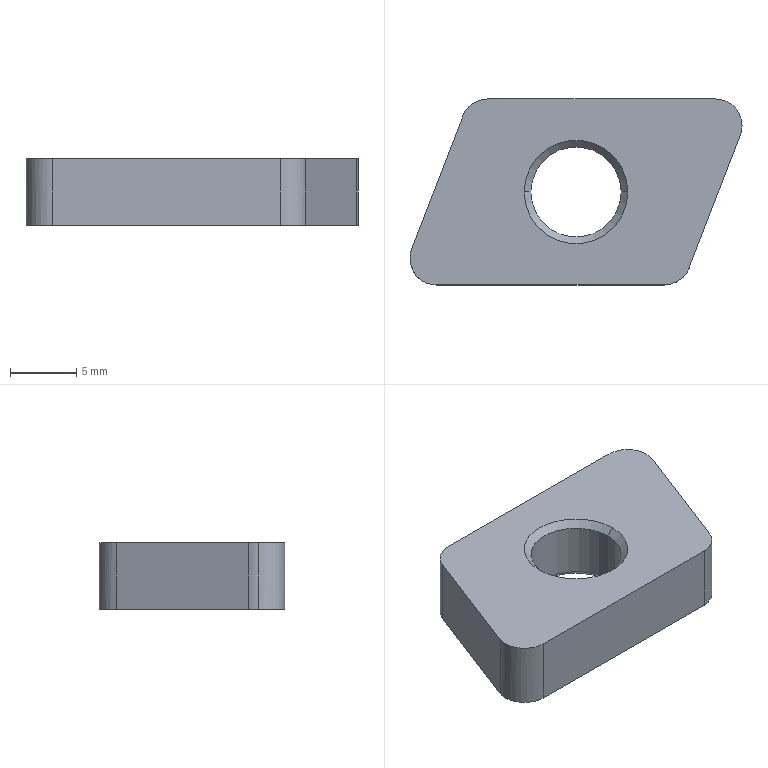Part | STEP file | 102000006924 | 1 solid | 18 faces | box 25 x 14 x 5 mm | volume 1290 mm3 | cylinder 8 | plane 6 | cone 4 | commonest cylinder face diameters 4 x6 6.8 x2
STEP:
#1=CARTESIAN_POINT('',(-2.355,42.772,4.5));
#2=VERTEX_POINT('',#1);
#3=CARTESIAN_POINT('',(4.445,42.772,4.5));
#4=VERTEX_POINT('',#3);
#5=CARTESIAN_POINT('',(1.045,42.772,4.5));
#6=DIRECTION('',(0.,0.,1.));
#7=AXIS2_PLACEMENT_3D('',#5,#6,$);
#8=CIRCLE('',#7,3.4);
#9=EDGE_CURVE('',#2,#4,#8,.T.);
#10=ORIENTED_EDGE('',*,*,#9,.F.);
#11=CARTESIAN_POINT('',(-2.855,42.772,5.));
#12=VERTEX_POINT('',#11);
#13=CARTESIAN_POINT('',(-353554.046,42.772,353556.191));
#14=DIRECTION('',(-0.7071,0.,0.7071));
#15=VECTOR('',#14,1.);
#16=LINE('',#13,#15);
#17=EDGE_CURVE('',#2,#12,#16,.T.);
#18=ORIENTED_EDGE('',*,*,#17,.T.);
#19=CARTESIAN_POINT('',(4.945,42.772,5.));
#20=VERTEX_POINT('',#19);
#21=CARTESIAN_POINT('',(1.045,42.772,5.));
#22=DIRECTION('',(0.,0.,1.));
#23=AXIS2_PLACEMENT_3D('',#21,#22,$);
#24=CIRCLE('',#23,3.9);
#25=EDGE_CURVE('',#20,#12,#24,.F.);
#26=ORIENTED_EDGE('',*,*,#25,.F.);
#27=CARTESIAN_POINT('',(353556.136,42.772,353556.191));
#28=DIRECTION('',(0.7071,0.,0.7071));
#29=VECTOR('',#28,1.);
#30=LINE('',#27,#29);
#31=EDGE_CURVE('',#4,#20,#30,.T.);
#32=ORIENTED_EDGE('',*,*,#31,.F.);
#33=EDGE_LOOP('',(#10,#18,#26,#32));
#34=FACE_OUTER_BOUND('',#33,.T.);
#35=CARTESIAN_POINT('',(1.045,42.772,4.5));
#36=DIRECTION('',(0.,0.,1.));
#37=DIRECTION('',(-1.,0.,0.));
#38=AXIS2_PLACEMENT_3D('',#35,#36,#37);
#39=CONICAL_SURFACE('',#38,3.4,0.7854);
#40=ADVANCED_FACE('',(#34),#39,.F.);
#41=CARTESIAN_POINT('',(4.445,42.772,0.5));
#42=VERTEX_POINT('',#41);
#43=CARTESIAN_POINT('',(-2.355,42.772,0.5));
#44=VERTEX_POINT('',#43);
#45=CARTESIAN_POINT('',(1.045,42.772,0.5));
#46=DIRECTION('',(0.,0.,1.));
#47=AXIS2_PLACEMENT_3D('',#45,#46,$);
#48=CIRCLE('',#47,3.4);
#49=EDGE_CURVE('',#42,#44,#48,.F.);
#50=ORIENTED_EDGE('',*,*,#49,.T.);
#51=CARTESIAN_POINT('',(-2.355,42.772,5.));
#52=DIRECTION('',(0.,0.,1.));
#53=VECTOR('',#52,1.);
#54=LINE('',#51,#53);
#55=EDGE_CURVE('',#44,#2,#54,.T.);
#56=ORIENTED_EDGE('',*,*,#55,.T.);
#57=ORIENTED_EDGE('',*,*,#9,.T.);
#58=CARTESIAN_POINT('',(4.445,42.772,5.));
#59=DIRECTION('',(0.,0.,1.));
#60=VECTOR('',#59,1.);
#61=LINE('',#58,#60);
#62=EDGE_CURVE('',#42,#4,#61,.T.);
#63=ORIENTED_EDGE('',*,*,#62,.F.);
#64=EDGE_LOOP('',(#50,#56,#57,#63));
#65=FACE_OUTER_BOUND('',#64,.T.);
#66=CARTESIAN_POINT('',(1.045,42.772,5.));
#67=DIRECTION('',(0.,0.,1.));
#68=DIRECTION('',(-1.,0.,0.));
#69=AXIS2_PLACEMENT_3D('',#66,#67,#68);
#70=CYLINDRICAL_SURFACE('',#69,3.4);
#71=ADVANCED_FACE('',(#65),#70,.F.);
#72=ORIENTED_EDGE('',*,*,#17,.F.);
#73=CARTESIAN_POINT('',(1.045,42.772,4.5));
#74=DIRECTION('',(0.,0.,1.));
#75=AXIS2_PLACEMENT_3D('',#73,#74,$);
#76=CIRCLE('',#75,3.4);
#77=EDGE_CURVE('',#4,#2,#76,.T.);
#78=ORIENTED_EDGE('',*,*,#77,.F.);
#79=ORIENTED_EDGE('',*,*,#31,.T.);
#80=CARTESIAN_POINT('',(1.045,42.772,5.));
#81=DIRECTION('',(0.,0.,1.));
#82=AXIS2_PLACEMENT_3D('',#80,#81,$);
#83=CIRCLE('',#82,3.9);
#84=EDGE_CURVE('',#12,#20,#83,.F.);
#85=ORIENTED_EDGE('',*,*,#84,.F.);
#86=EDGE_LOOP('',(#72,#78,#79,#85));
#87=FACE_OUTER_BOUND('',#86,.T.);
#88=CARTESIAN_POINT('',(1.045,42.772,4.5));
#89=DIRECTION('',(0.,0.,1.));
#90=DIRECTION('',(1.,0.,0.));
#91=AXIS2_PLACEMENT_3D('',#88,#89,#90);
#92=CONICAL_SURFACE('',#91,3.4,0.7854);
#93=ADVANCED_FACE('',(#87),#92,.F.);
#94=CARTESIAN_POINT('',(-9.455,35.772,5.));
#95=VERTEX_POINT('',#94);
#96=CARTESIAN_POINT('',(7.692,35.772,5.));
#97=VERTEX_POINT('',#96);
#98=CARTESIAN_POINT('',(-0.8816,35.772,5.));
#99=DIRECTION('',(1.,0.,0.));
#100=VECTOR('',#99,1.);
#101=LINE('',#98,#100);
#102=EDGE_CURVE('',#95,#97,#101,.T.);
#103=ORIENTED_EDGE('',*,*,#102,.T.);
#104=CARTESIAN_POINT('',(9.558,37.053,5.));
#105=VERTEX_POINT('',#104);
#106=CARTESIAN_POINT('',(7.692,35.772,5.));
#107=CARTESIAN_POINT('',(7.9,35.772,5.));
#108=CARTESIAN_POINT('',(8.107,35.799,5.));
#109=CARTESIAN_POINT('',(8.311,35.853,5.));
#110=CARTESIAN_POINT('',(8.698,36.012,5.));
#111=CARTESIAN_POINT('',(9.032,36.266,5.));
#112=CARTESIAN_POINT('',(9.182,36.413,5.));
#113=CARTESIAN_POINT('',(9.351,36.631,5.));
#114=CARTESIAN_POINT('',(9.48,36.872,5.));
#115=CARTESIAN_POINT('',(9.508,36.931,5.));
#116=CARTESIAN_POINT('',(9.534,36.991,5.));
#117=CARTESIAN_POINT('',(9.558,37.053,5.));
#118=B_SPLINE_CURVE_WITH_KNOTS('',5,(#106,#107,#108,#109,#110,#111,#112,#113,#114,#115,#116,#117),.UNSPECIFIED.,.F.,.U.,(6,3,3,6),(0.,1.47,2.939,3.402),.UNSPECIFIED.);
#119=EDGE_CURVE('',#97,#105,#118,.T.);
#120=ORIENTED_EDGE('',*,*,#119,.T.);
#121=CARTESIAN_POINT('',(13.411,47.053,5.));
#122=VERTEX_POINT('',#121);
#123=CARTESIAN_POINT('',(11.485,42.053,5.));
#124=DIRECTION('',(0.3596,0.9331,0.));
#125=VECTOR('',#124,1.);
#126=LINE('',#123,#125);
#127=EDGE_CURVE('',#105,#122,#126,.T.);
#128=ORIENTED_EDGE('',*,*,#127,.T.);
#129=CARTESIAN_POINT('',(13.545,47.772,5.));
#130=VERTEX_POINT('',#129);
#131=CARTESIAN_POINT('',(13.411,47.053,5.));
#132=CARTESIAN_POINT('',(13.464,47.19,5.));
#133=CARTESIAN_POINT('',(13.504,47.332,5.));
#134=CARTESIAN_POINT('',(13.531,47.477,5.));
#135=CARTESIAN_POINT('',(13.545,47.625,5.));
#136=CARTESIAN_POINT('',(13.545,47.772,5.));
#137=B_SPLINE_CURVE_WITH_KNOTS('',5,(#131,#132,#133,#134,#135,#136),.UNSPECIFIED.,.F.,.U.,(6,6),(0.,1.04),.UNSPECIFIED.);
#138=EDGE_CURVE('',#122,#130,#137,.T.);
#139=ORIENTED_EDGE('',*,*,#138,.T.);
#140=CARTESIAN_POINT('',(11.545,49.772,5.));
#141=VERTEX_POINT('',#140);
#142=CARTESIAN_POINT('',(13.545,47.772,5.));
#143=CARTESIAN_POINT('',(13.545,47.832,5.));
#144=CARTESIAN_POINT('',(13.543,47.893,5.));
#145=CARTESIAN_POINT('',(13.538,47.954,5.));
#146=CARTESIAN_POINT('',(13.508,48.221,5.));
#147=CARTESIAN_POINT('',(13.432,48.481,5.));
#148=CARTESIAN_POINT('',(13.348,48.674,5.));
#149=CARTESIAN_POINT('',(13.132,49.033,5.));
#150=CARTESIAN_POINT('',(12.831,49.325,5.));
#151=CARTESIAN_POINT('',(12.662,49.45,5.));
#152=CARTESIAN_POINT('',(12.346,49.627,5.));
#153=CARTESIAN_POINT('',(11.999,49.728,5.));
#154=CARTESIAN_POINT('',(11.849,49.757,5.));
#155=CARTESIAN_POINT('',(11.697,49.772,5.));
#156=CARTESIAN_POINT('',(11.545,49.772,5.));
#157=B_SPLINE_CURVE_WITH_KNOTS('',5,(#142,#143,#144,#145,#146,#147,#148,#149,#150,#151,#152,#153,#154,#155,#156),.UNSPECIFIED.,.F.,.U.,(6,3,3,3,6),(1.04,1.47,2.939,4.409,5.483),.UNSPECIFIED.);
#158=EDGE_CURVE('',#130,#141,#157,.T.);
#159=ORIENTED_EDGE('',*,*,#158,.T.);
#160=CARTESIAN_POINT('',(-5.602,49.772,5.));
#161=VERTEX_POINT('',#160);
#162=CARTESIAN_POINT('',(2.972,49.772,5.));
#163=DIRECTION('',(-1.,0.,0.));
#164=VECTOR('',#163,1.);
#165=LINE('',#162,#164);
#166=EDGE_CURVE('',#141,#161,#165,.T.);
#167=ORIENTED_EDGE('',*,*,#166,.T.);
#168=CARTESIAN_POINT('',(-7.468,48.491,5.));
#169=VERTEX_POINT('',#168);
#170=CARTESIAN_POINT('',(-5.602,49.772,5.));
#171=CARTESIAN_POINT('',(-5.81,49.772,5.));
#172=CARTESIAN_POINT('',(-6.017,49.745,5.));
#173=CARTESIAN_POINT('',(-6.221,49.691,5.));
#174=CARTESIAN_POINT('',(-6.608,49.531,5.));
#175=CARTESIAN_POINT('',(-6.942,49.278,5.));
#176=CARTESIAN_POINT('',(-7.092,49.13,5.));
#177=CARTESIAN_POINT('',(-7.261,48.912,5.));
#178=CARTESIAN_POINT('',(-7.39,48.671,5.));
#179=CARTESIAN_POINT('',(-7.418,48.612,5.));
#180=CARTESIAN_POINT('',(-7.444,48.552,5.));
#181=CARTESIAN_POINT('',(-7.468,48.491,5.));
#182=B_SPLINE_CURVE_WITH_KNOTS('',5,(#170,#171,#172,#173,#174,#175,#176,#177,#178,#179,#180,#181),.UNSPECIFIED.,.F.,.U.,(6,3,3,6),(0.,1.47,2.939,3.402),.UNSPECIFIED.);
#183=EDGE_CURVE('',#161,#169,#182,.T.);
#184=ORIENTED_EDGE('',*,*,#183,.T.);
#185=CARTESIAN_POINT('',(-11.321,38.491,5.));
#186=VERTEX_POINT('',#185);
#187=CARTESIAN_POINT('',(-9.395,43.491,5.));
#188=DIRECTION('',(-0.3596,-0.9331,0.));
#189=VECTOR('',#188,1.);
#190=LINE('',#187,#189);
#191=EDGE_CURVE('',#169,#186,#190,.T.);
#192=ORIENTED_EDGE('',*,*,#191,.T.);
#193=CARTESIAN_POINT('',(-11.455,37.772,5.));
#194=VERTEX_POINT('',#193);
#195=CARTESIAN_POINT('',(-11.321,38.491,5.));
#196=CARTESIAN_POINT('',(-11.374,38.354,5.));
#197=CARTESIAN_POINT('',(-11.414,38.211,5.));
#198=CARTESIAN_POINT('',(-11.441,38.066,5.));
#199=CARTESIAN_POINT('',(-11.455,37.919,5.));
#200=CARTESIAN_POINT('',(-11.455,37.772,5.));
#201=B_SPLINE_CURVE_WITH_KNOTS('',5,(#195,#196,#197,#198,#199,#200),.UNSPECIFIED.,.F.,.U.,(6,6),(0.,1.04),.UNSPECIFIED.);
#202=EDGE_CURVE('',#186,#194,#201,.T.);
#203=ORIENTED_EDGE('',*,*,#202,.T.);
#204=CARTESIAN_POINT('',(-11.455,37.772,5.));
#205=CARTESIAN_POINT('',(-11.455,37.564,5.));
#206=CARTESIAN_POINT('',(-11.428,37.356,5.));
#207=CARTESIAN_POINT('',(-11.374,37.153,5.));
#208=CARTESIAN_POINT('',(-11.214,36.765,5.));
#209=CARTESIAN_POINT('',(-10.961,36.431,5.));
#210=CARTESIAN_POINT('',(-10.813,36.282,5.));
#211=CARTESIAN_POINT('',(-10.482,36.024,5.));
#212=CARTESIAN_POINT('',(-10.097,35.86,5.));
#213=CARTESIAN_POINT('',(-9.894,35.804,5.));
#214=CARTESIAN_POINT('',(-9.682,35.774,5.));
#215=CARTESIAN_POINT('',(-9.469,35.772,5.));
#216=CARTESIAN_POINT('',(-9.465,35.772,5.));
#217=CARTESIAN_POINT('',(-9.46,35.772,5.));
#218=CARTESIAN_POINT('',(-9.455,35.772,5.));
#219=B_SPLINE_CURVE_WITH_KNOTS('',5,(#204,#205,#206,#207,#208,#209,#210,#211,#212,#213,#214,#215,#216,#217,#218),.UNSPECIFIED.,.F.,.U.,(6,3,3,3,6),(0.,1.47,2.939,4.409,4.443),.UNSPECIFIED.);
#220=EDGE_CURVE('',#194,#95,#219,.T.);
#221=ORIENTED_EDGE('',*,*,#220,.T.);
#222=EDGE_LOOP('',(#103,#120,#128,#139,#159,#167,#184,#192,#203,#221));
#223=FACE_OUTER_BOUND('',#222,.T.);
#224=ORIENTED_EDGE('',*,*,#25,.T.);
#225=ORIENTED_EDGE('',*,*,#84,.T.);
#226=EDGE_LOOP('',(#224,#225));
#227=FACE_BOUND('',#226,.T.);
#228=CARTESIAN_POINT('',(11.545,47.772,5.));
#229=DIRECTION('',(0.,0.,-1.));
#230=DIRECTION('',(-1.,0.,0.));
#231=AXIS2_PLACEMENT_3D('',#228,#229,#230);
#232=PLANE('',#231);
#233=ADVANCED_FACE('',(#223,#227),#232,.F.);
#234=ORIENTED_EDGE('',*,*,#49,.F.);
#235=CARTESIAN_POINT('',(4.945,42.772,0.));
#236=VERTEX_POINT('',#235);
#237=CARTESIAN_POINT('',(353556.136,42.772,-353551.191));
#238=DIRECTION('',(0.7071,0.,-0.7071));
#239=VECTOR('',#238,1.);
#240=LINE('',#237,#239);
#241=EDGE_CURVE('',#42,#236,#240,.T.);
#242=ORIENTED_EDGE('',*,*,#241,.T.);
#243=CARTESIAN_POINT('',(-2.855,42.772,0.));
#244=VERTEX_POINT('',#243);
#245=CARTESIAN_POINT('',(1.045,42.772,0.));
#246=DIRECTION('',(0.,0.,-1.));
#247=AXIS2_PLACEMENT_3D('',#245,#246,$);
#248=CIRCLE('',#247,3.9);
#249=EDGE_CURVE('',#244,#236,#248,.F.);
#250=ORIENTED_EDGE('',*,*,#249,.F.);
#251=CARTESIAN_POINT('',(-353554.046,42.772,-353551.191));
#252=DIRECTION('',(-0.7071,0.,-0.7071));
#253=VECTOR('',#252,1.);
#254=LINE('',#251,#253);
#255=EDGE_CURVE('',#44,#244,#254,.T.);
#256=ORIENTED_EDGE('',*,*,#255,.F.);
#257=EDGE_LOOP('',(#234,#242,#250,#256));
#258=FACE_OUTER_BOUND('',#257,.T.);
#259=CARTESIAN_POINT('',(1.045,42.772,0.5));
#260=DIRECTION('',(0.,0.,-1.));
#261=DIRECTION('',(1.,0.,0.));
#262=AXIS2_PLACEMENT_3D('',#259,#260,#261);
#263=CONICAL_SURFACE('',#262,3.4,0.7854);
#264=ADVANCED_FACE('',(#258),#263,.F.);
#265=ORIENTED_EDGE('',*,*,#55,.F.);
#266=CARTESIAN_POINT('',(1.045,42.772,0.5));
#267=DIRECTION('',(0.,0.,1.));
#268=AXIS2_PLACEMENT_3D('',#266,#267,$);
#269=CIRCLE('',#268,3.4);
#270=EDGE_CURVE('',#44,#42,#269,.F.);
#271=ORIENTED_EDGE('',*,*,#270,.T.);
#272=ORIENTED_EDGE('',*,*,#62,.T.);
#273=ORIENTED_EDGE('',*,*,#77,.T.);
#274=EDGE_LOOP('',(#265,#271,#272,#273));
#275=FACE_OUTER_BOUND('',#274,.T.);
#276=CARTESIAN_POINT('',(1.045,42.772,5.));
#277=DIRECTION('',(0.,0.,1.));
#278=DIRECTION('',(1.,0.,0.));
#279=AXIS2_PLACEMENT_3D('',#276,#277,#278);
#280=CYLINDRICAL_SURFACE('',#279,3.4);
#281=ADVANCED_FACE('',(#275),#280,.F.);
#282=CARTESIAN_POINT('',(-9.455,35.772,0.));
#283=VERTEX_POINT('',#282);
#284=CARTESIAN_POINT('',(7.692,35.772,0.));
#285=VERTEX_POINT('',#284);
#286=CARTESIAN_POINT('',(-0.8816,35.772,0.));
#287=DIRECTION('',(1.,0.,0.));
#288=VECTOR('',#287,1.);
#289=LINE('',#286,#288);
#290=EDGE_CURVE('',#283,#285,#289,.T.);
#291=ORIENTED_EDGE('',*,*,#290,.T.);
#292=CARTESIAN_POINT('',(7.692,35.772,2.5));
#293=DIRECTION('',(0.,0.,1.));
#294=VECTOR('',#293,1.);
#295=LINE('',#292,#294);
#296=EDGE_CURVE('',#285,#97,#295,.T.);
#297=ORIENTED_EDGE('',*,*,#296,.T.);
#298=ORIENTED_EDGE('',*,*,#102,.F.);
#299=CARTESIAN_POINT('',(-9.455,35.772,2.5));
#300=DIRECTION('',(0.,0.,-1.));
#301=VECTOR('',#300,1.);
#302=LINE('',#299,#301);
#303=EDGE_CURVE('',#95,#283,#302,.T.);
#304=ORIENTED_EDGE('',*,*,#303,.T.);
#305=EDGE_LOOP('',(#291,#297,#298,#304));
#306=FACE_OUTER_BOUND('',#305,.T.);
#307=CARTESIAN_POINT('',(-9.455,35.772,5.));
#308=DIRECTION('',(0.,1.,0.));
#309=DIRECTION('',(0.,0.,1.));
#310=AXIS2_PLACEMENT_3D('',#307,#308,#309);
#311=PLANE('',#310);
#312=ADVANCED_FACE('',(#306),#311,.F.);
#313=ORIENTED_EDGE('',*,*,#119,.F.);
#314=ORIENTED_EDGE('',*,*,#296,.F.);
#315=CARTESIAN_POINT('',(9.558,37.053,0.));
#316=VERTEX_POINT('',#315);
#317=CARTESIAN_POINT('',(7.692,37.772,0.));
#318=DIRECTION('',(0.,0.,-1.));
#319=AXIS2_PLACEMENT_3D('',#317,#318,$);
#320=CIRCLE('',#319,2.);
#321=EDGE_CURVE('',#316,#285,#320,.T.);
#322=ORIENTED_EDGE('',*,*,#321,.F.);
#323=CARTESIAN_POINT('',(9.558,37.053,5.));
#324=DIRECTION('',(0.,0.,-1.));
#325=VECTOR('',#324,1.);
#326=LINE('',#323,#325);
#327=EDGE_CURVE('',#105,#316,#326,.T.);
#328=ORIENTED_EDGE('',*,*,#327,.F.);
#329=EDGE_LOOP('',(#313,#314,#322,#328));
#330=FACE_OUTER_BOUND('',#329,.T.);
#331=CARTESIAN_POINT('',(7.692,37.772,5.));
#332=DIRECTION('',(0.,0.,-1.));
#333=DIRECTION('',(1.,0.,0.));
#334=AXIS2_PLACEMENT_3D('',#331,#332,#333);
#335=CYLINDRICAL_SURFACE('',#334,2.);
#336=ADVANCED_FACE('',(#330),#335,.T.);
#337=ORIENTED_EDGE('',*,*,#127,.F.);
#338=ORIENTED_EDGE('',*,*,#327,.T.);
#339=CARTESIAN_POINT('',(13.411,47.053,0.));
#340=VERTEX_POINT('',#339);
#341=CARTESIAN_POINT('',(11.485,42.053,0.));
#342=DIRECTION('',(0.3596,0.9331,0.));
#343=VECTOR('',#342,1.);
#344=LINE('',#341,#343);
#345=EDGE_CURVE('',#316,#340,#344,.T.);
#346=ORIENTED_EDGE('',*,*,#345,.T.);
#347=CARTESIAN_POINT('',(13.411,47.053,2.5));
#348=DIRECTION('',(0.,0.,-1.));
#349=VECTOR('',#348,1.);
#350=LINE('',#347,#349);
#351=EDGE_CURVE('',#122,#340,#350,.T.);
#352=ORIENTED_EDGE('',*,*,#351,.F.);
#353=EDGE_LOOP('',(#337,#338,#346,#352));
#354=FACE_OUTER_BOUND('',#353,.T.);
#355=CARTESIAN_POINT('',(9.064,35.772,5.));
#356=DIRECTION('',(-0.9331,0.3596,0.));
#357=DIRECTION('',(-0.3596,-0.9331,0.));
#358=AXIS2_PLACEMENT_3D('',#355,#356,#357);
#359=PLANE('',#358);
#360=ADVANCED_FACE('',(#354),#359,.F.);
#361=CARTESIAN_POINT('',(13.545,47.772,0.));
#362=VERTEX_POINT('',#361);
#363=CARTESIAN_POINT('',(13.545,47.772,5.));
#364=DIRECTION('',(0.,0.,-1.));
#365=VECTOR('',#364,1.);
#366=LINE('',#363,#365);
#367=EDGE_CURVE('',#130,#362,#366,.T.);
#368=ORIENTED_EDGE('',*,*,#367,.F.);
#369=ORIENTED_EDGE('',*,*,#138,.F.);
#370=ORIENTED_EDGE('',*,*,#351,.T.);
#371=CARTESIAN_POINT('',(11.545,47.772,0.));
#372=DIRECTION('',(0.,0.,-1.));
#373=AXIS2_PLACEMENT_3D('',#371,#372,$);
#374=CIRCLE('',#373,2.);
#375=EDGE_CURVE('',#340,#362,#374,.F.);
#376=ORIENTED_EDGE('',*,*,#375,.T.);
#377=EDGE_LOOP('',(#368,#369,#370,#376));
#378=FACE_OUTER_BOUND('',#377,.T.);
#379=CARTESIAN_POINT('',(11.545,47.772,5.));
#380=DIRECTION('',(0.,0.,-1.));
#381=DIRECTION('',(1.,0.,0.));
#382=AXIS2_PLACEMENT_3D('',#379,#380,#381);
#383=CYLINDRICAL_SURFACE('',#382,2.);
#384=ADVANCED_FACE('',(#378),#383,.T.);
#385=ORIENTED_EDGE('',*,*,#367,.T.);
#386=CARTESIAN_POINT('',(11.545,49.772,0.));
#387=VERTEX_POINT('',#386);
#388=CARTESIAN_POINT('',(11.545,47.772,0.));
#389=DIRECTION('',(0.,0.,-1.));
#390=AXIS2_PLACEMENT_3D('',#388,#389,$);
#391=CIRCLE('',#390,2.);
#392=EDGE_CURVE('',#362,#387,#391,.F.);
#393=ORIENTED_EDGE('',*,*,#392,.T.);
#394=CARTESIAN_POINT('',(11.545,49.772,5.));
#395=DIRECTION('',(0.,0.,-1.));
#396=VECTOR('',#395,1.);
#397=LINE('',#394,#396);
#398=EDGE_CURVE('',#141,#387,#397,.T.);
#399=ORIENTED_EDGE('',*,*,#398,.F.);
#400=ORIENTED_EDGE('',*,*,#158,.F.);
#401=EDGE_LOOP('',(#385,#393,#399,#400));
#402=FACE_OUTER_BOUND('',#401,.T.);
#403=CARTESIAN_POINT('',(11.545,47.772,5.));
#404=DIRECTION('',(0.,0.,-1.));
#405=DIRECTION('',(-1.,0.,0.));
#406=AXIS2_PLACEMENT_3D('',#403,#404,#405);
#407=CYLINDRICAL_SURFACE('',#406,2.);
#408=ADVANCED_FACE('',(#402),#407,.T.);
#409=CARTESIAN_POINT('',(-5.602,49.772,0.));
#410=VERTEX_POINT('',#409);
#411=CARTESIAN_POINT('',(2.972,49.772,0.));
#412=DIRECTION('',(-1.,0.,0.));
#413=VECTOR('',#412,1.);
#414=LINE('',#411,#413);
#415=EDGE_CURVE('',#387,#410,#414,.T.);
#416=ORIENTED_EDGE('',*,*,#415,.T.);
#417=CARTESIAN_POINT('',(-5.602,49.772,2.5));
#418=DIRECTION('',(0.,0.,1.));
#419=VECTOR('',#418,1.);
#420=LINE('',#417,#419);
#421=EDGE_CURVE('',#410,#161,#420,.T.);
#422=ORIENTED_EDGE('',*,*,#421,.T.);
#423=ORIENTED_EDGE('',*,*,#166,.F.);
#424=ORIENTED_EDGE('',*,*,#398,.T.);
#425=EDGE_LOOP('',(#416,#422,#423,#424));
#426=FACE_OUTER_BOUND('',#425,.T.);
#427=CARTESIAN_POINT('',(-6.974,49.772,5.));
#428=DIRECTION('',(0.,-1.,0.));
#429=DIRECTION('',(1.,0.,0.));
#430=AXIS2_PLACEMENT_3D('',#427,#428,#429);
#431=PLANE('',#430);
#432=ADVANCED_FACE('',(#426),#431,.F.);
#433=ORIENTED_EDGE('',*,*,#183,.F.);
#434=ORIENTED_EDGE('',*,*,#421,.F.);
#435=CARTESIAN_POINT('',(-7.468,48.491,0.));
#436=VERTEX_POINT('',#435);
#437=CARTESIAN_POINT('',(-5.602,47.772,0.));
#438=DIRECTION('',(0.,0.,-1.));
#439=AXIS2_PLACEMENT_3D('',#437,#438,$);
#440=CIRCLE('',#439,2.);
#441=EDGE_CURVE('',#436,#410,#440,.T.);
#442=ORIENTED_EDGE('',*,*,#441,.F.);
#443=CARTESIAN_POINT('',(-7.468,48.491,5.));
#444=DIRECTION('',(0.,0.,-1.));
#445=VECTOR('',#444,1.);
#446=LINE('',#443,#445);
#447=EDGE_CURVE('',#169,#436,#446,.T.);
#448=ORIENTED_EDGE('',*,*,#447,.F.);
#449=EDGE_LOOP('',(#433,#434,#442,#448));
#450=FACE_OUTER_BOUND('',#449,.T.);
#451=CARTESIAN_POINT('',(-5.602,47.772,5.));
#452=DIRECTION('',(0.,0.,-1.));
#453=DIRECTION('',(-1.,0.,0.));
#454=AXIS2_PLACEMENT_3D('',#451,#452,#453);
#455=CYLINDRICAL_SURFACE('',#454,2.);
#456=ADVANCED_FACE('',(#450),#455,.T.);
#457=ORIENTED_EDGE('',*,*,#191,.F.);
#458=ORIENTED_EDGE('',*,*,#447,.T.);
#459=CARTESIAN_POINT('',(-11.321,38.491,0.));
#460=VERTEX_POINT('',#459);
#461=CARTESIAN_POINT('',(-9.395,43.491,0.));
#462=DIRECTION('',(-0.3596,-0.9331,0.));
#463=VECTOR('',#462,1.);
#464=LINE('',#461,#463);
#465=EDGE_CURVE('',#436,#460,#464,.T.);
#466=ORIENTED_EDGE('',*,*,#465,.T.);
#467=CARTESIAN_POINT('',(-11.321,38.491,2.5));
#468=DIRECTION('',(0.,0.,-1.));
#469=VECTOR('',#468,1.);
#470=LINE('',#467,#469);
#471=EDGE_CURVE('',#186,#460,#470,.T.);
#472=ORIENTED_EDGE('',*,*,#471,.F.);
#473=EDGE_LOOP('',(#457,#458,#466,#472));
#474=FACE_OUTER_BOUND('',#473,.T.);
#475=CARTESIAN_POINT('',(-11.321,38.491,5.));
#476=DIRECTION('',(0.9331,-0.3596,0.));
#477=DIRECTION('',(0.3596,0.9331,0.));
#478=AXIS2_PLACEMENT_3D('',#475,#476,#477);
#479=PLANE('',#478);
#480=ADVANCED_FACE('',(#474),#479,.F.);
#481=CARTESIAN_POINT('',(-11.455,37.772,0.));
#482=VERTEX_POINT('',#481);
#483=CARTESIAN_POINT('',(-11.455,37.772,5.));
#484=DIRECTION('',(0.,0.,-1.));
#485=VECTOR('',#484,1.);
#486=LINE('',#483,#485);
#487=EDGE_CURVE('',#194,#482,#486,.T.);
#488=ORIENTED_EDGE('',*,*,#487,.F.);
#489=ORIENTED_EDGE('',*,*,#202,.F.);
#490=ORIENTED_EDGE('',*,*,#471,.T.);
#491=CARTESIAN_POINT('',(-9.455,37.772,0.));
#492=DIRECTION('',(0.,0.,-1.));
#493=AXIS2_PLACEMENT_3D('',#491,#492,$);
#494=CIRCLE('',#493,2.);
#495=EDGE_CURVE('',#460,#482,#494,.F.);
#496=ORIENTED_EDGE('',*,*,#495,.T.);
#497=EDGE_LOOP('',(#488,#489,#490,#496));
#498=FACE_OUTER_BOUND('',#497,.T.);
#499=CARTESIAN_POINT('',(-9.455,37.772,5.));
#500=DIRECTION('',(0.,0.,-1.));
#501=DIRECTION('',(-1.,0.,0.));
#502=AXIS2_PLACEMENT_3D('',#499,#500,#501);
#503=CYLINDRICAL_SURFACE('',#502,2.);
#504=ADVANCED_FACE('',(#498),#503,.T.);
#505=ORIENTED_EDGE('',*,*,#220,.F.);
#506=ORIENTED_EDGE('',*,*,#487,.T.);
#507=CARTESIAN_POINT('',(-9.455,37.772,0.));
#508=DIRECTION('',(0.,0.,-1.));
#509=AXIS2_PLACEMENT_3D('',#507,#508,$);
#510=CIRCLE('',#509,2.);
#511=EDGE_CURVE('',#482,#283,#510,.F.);
#512=ORIENTED_EDGE('',*,*,#511,.T.);
#513=ORIENTED_EDGE('',*,*,#303,.F.);
#514=EDGE_LOOP('',(#505,#506,#512,#513));
#515=FACE_OUTER_BOUND('',#514,.T.);
#516=CARTESIAN_POINT('',(-9.455,37.772,5.));
#517=DIRECTION('',(0.,0.,-1.));
#518=DIRECTION('',(1.,0.,0.));
#519=AXIS2_PLACEMENT_3D('',#516,#517,#518);
#520=CYLINDRICAL_SURFACE('',#519,2.);
#521=ADVANCED_FACE('',(#515),#520,.T.);
#522=ORIENTED_EDGE('',*,*,#241,.F.);
#523=ORIENTED_EDGE('',*,*,#270,.F.);
#524=ORIENTED_EDGE('',*,*,#255,.T.);
#525=CARTESIAN_POINT('',(1.045,42.772,0.));
#526=DIRECTION('',(0.,0.,-1.));
#527=AXIS2_PLACEMENT_3D('',#525,#526,$);
#528=CIRCLE('',#527,3.9);
#529=EDGE_CURVE('',#236,#244,#528,.F.);
#530=ORIENTED_EDGE('',*,*,#529,.F.);
#531=EDGE_LOOP('',(#522,#523,#524,#530));
#532=FACE_OUTER_BOUND('',#531,.T.);
#533=CARTESIAN_POINT('',(1.045,42.772,0.5));
#534=DIRECTION('',(0.,0.,-1.));
#535=DIRECTION('',(-1.,0.,0.));
#536=AXIS2_PLACEMENT_3D('',#533,#534,#535);
#537=CONICAL_SURFACE('',#536,3.4,0.7854);
#538=ADVANCED_FACE('',(#532),#537,.F.);
#539=ORIENTED_EDGE('',*,*,#345,.F.);
#540=ORIENTED_EDGE('',*,*,#321,.T.);
#541=ORIENTED_EDGE('',*,*,#290,.F.);
#542=ORIENTED_EDGE('',*,*,#511,.F.);
#543=ORIENTED_EDGE('',*,*,#495,.F.);
#544=ORIENTED_EDGE('',*,*,#465,.F.);
#545=ORIENTED_EDGE('',*,*,#441,.T.);
#546=ORIENTED_EDGE('',*,*,#415,.F.);
#547=ORIENTED_EDGE('',*,*,#392,.F.);
#548=ORIENTED_EDGE('',*,*,#375,.F.);
#549=EDGE_LOOP('',(#539,#540,#541,#542,#543,#544,#545,#546,#547,#548));
#550=FACE_OUTER_BOUND('',#549,.T.);
#551=ORIENTED_EDGE('',*,*,#249,.T.);
#552=ORIENTED_EDGE('',*,*,#529,.T.);
#553=EDGE_LOOP('',(#551,#552));
#554=FACE_BOUND('',#553,.T.);
#555=CARTESIAN_POINT('',(11.545,47.772,0.));
#556=DIRECTION('',(0.,0.,-1.));
#557=DIRECTION('',(-1.,0.,0.));
#558=AXIS2_PLACEMENT_3D('',#555,#556,#557);
#559=PLANE('',#558);
#560=ADVANCED_FACE('',(#550,#554),#559,.T.);
#561=CLOSED_SHELL('',(#40,#71,#93,#233,#264,#281,#312,#336,#360,#384,#408,#432,#456,#480,#504,#521,#538,#560));
#562=MANIFOLD_SOLID_BREP('',#561);
#563=(LENGTH_UNIT()NAMED_UNIT(*)SI_UNIT(.MILLI.,.METRE.));
#564=UNCERTAINTY_MEASURE_WITH_UNIT(LENGTH_MEASURE(0.005),#563,'','');
#565=(NAMED_UNIT(*)PLANE_ANGLE_UNIT()SI_UNIT($,.RADIAN.));
#566=(NAMED_UNIT(*)SI_UNIT($,.STERADIAN.)SOLID_ANGLE_UNIT());
#567=(GEOMETRIC_REPRESENTATION_CONTEXT(3)GLOBAL_UNCERTAINTY_ASSIGNED_CONTEXT((#564))GLOBAL_UNIT_ASSIGNED_CONTEXT((#563,#565,#566))REPRESENTATION_CONTEXT('',''));
#568=ADVANCED_BREP_SHAPE_REPRESENTATION('',(#562),#567);